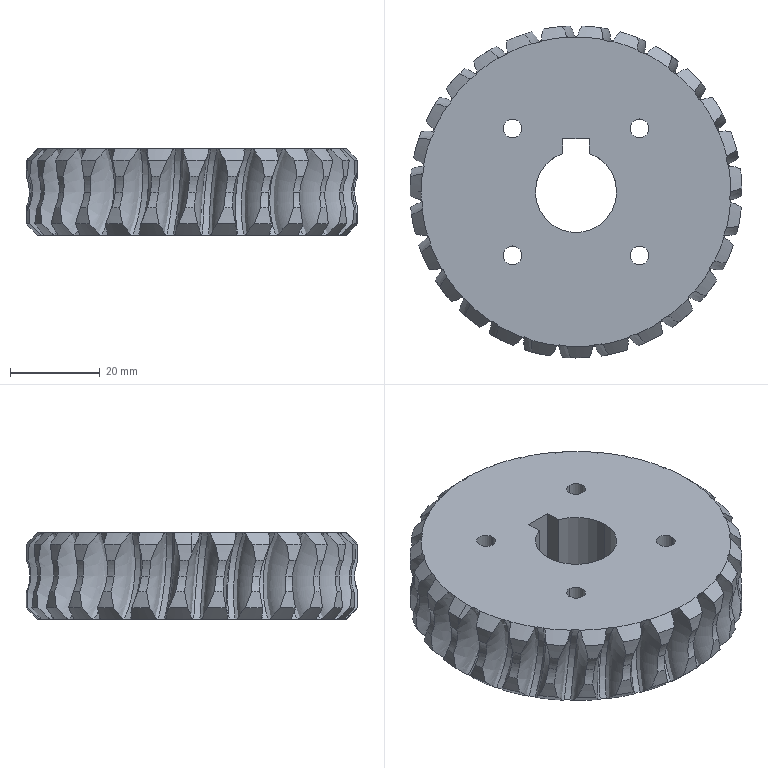Part | SolidWorks | features CirPattern 2, Cut 1, Helix 1, HoleWzd 1, RefAxis 1, Revolution 1, SweepCut 1 | 1 solid | 262 faces | box 73.955 x 73.932 x 19.18 mm | volume 65019 mm3 | spline 81 | cylinder 66 | cone 56 | torus 54 | plane 5 | commonest cylinder face diameters 73.955 x55 4.2 x8 18.125 x3